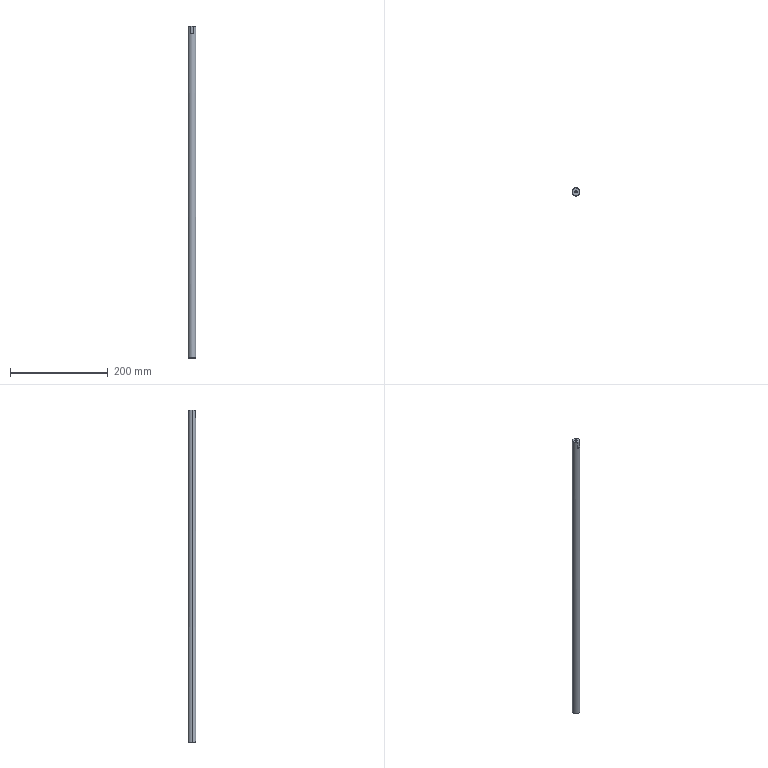Part | STEP file | Support Shaft | 1 solid | 17 faces | box 16 x 16 x 680 mm | volume 136250 mm3 | cone 7 | plane 6 | cylinder 4 | commonest cylinder face diameters 5 x2 16 x2
STEP:
#1=CARTESIAN_POINT('',(0.,0.,0.));
#2=DIRECTION('',(0.,0.,1.));
#3=DIRECTION('',(1.,0.,0.));
#4=AXIS2_PLACEMENT_3D('',#1,#2,#3);
#5=CARTESIAN_POINT('',(-7.5,0.,0.));
#6=VERTEX_POINT('',#5);
#7=CARTESIAN_POINT('',(7.5,0.,0.));
#8=VERTEX_POINT('',#7);
#9=CARTESIAN_POINT('',(0.,0.,0.));
#10=DIRECTION('',(0.,0.,-1.));
#11=DIRECTION('',(1.,0.,0.));
#12=AXIS2_PLACEMENT_3D('',#9,#10,#11);
#13=CIRCLE('',#12,7.5);
#14=CARTESIAN_POINT('',(0.,0.,0.5));
#15=DIRECTION('',(0.,0.,1.));
#16=DIRECTION('',(1.,0.,0.));
#17=AXIS2_PLACEMENT_3D('',#14,#15,#16);
#18=CONICAL_SURFACE('',#17,8.,0.7854);
#19=CARTESIAN_POINT('',(6.283,-0.5));
#20=DIRECTION('',(-1.,0.));
#21=VECTOR('',#20,1.);
#22=LINE('',#19,#21);
#23=(GEOMETRIC_REPRESENTATION_CONTEXT(2)PARAMETRIC_REPRESENTATION_CONTEXT()REPRESENTATION_CONTEXT('',''));
#24=DEFINITIONAL_REPRESENTATION('',(#22),#23);
#25=PCURVE('',#18,#24);
#26=CARTESIAN_POINT('',(0.,0.,0.));
#27=DIRECTION('',(0.,0.,1.));
#28=DIRECTION('',(1.,0.,0.));
#29=AXIS2_PLACEMENT_3D('',#26,#27,#28);
#30=PLANE('',#29);
#31=CARTESIAN_POINT('',(7.5,0.));
#32=CARTESIAN_POINT('',(7.5,-12.99));
#33=CARTESIAN_POINT('',(-3.75,-6.495));
#34=CARTESIAN_POINT('',(-15.,0.));
#35=CARTESIAN_POINT('',(-3.75,6.495));
#36=CARTESIAN_POINT('',(7.5,12.99));
#37=CARTESIAN_POINT('',(7.5,0.));
#38=(BOUNDED_CURVE()B_SPLINE_CURVE(2,(#31,#32,#33,#34,#35,#36,#37),.UNSPECIFIED.,.T.,.F.)B_SPLINE_CURVE_WITH_KNOTS((1,2,2,2,2,1),(-2.094,0.,2.094,4.189,6.283,8.378),.UNSPECIFIED.)CURVE()GEOMETRIC_REPRESENTATION_ITEM()RATIONAL_B_SPLINE_CURVE((1.,0.5,1.,0.5,1.,0.5,1.))REPRESENTATION_ITEM(''));
#39=(GEOMETRIC_REPRESENTATION_CONTEXT(2)PARAMETRIC_REPRESENTATION_CONTEXT()REPRESENTATION_CONTEXT('',''));
#40=DEFINITIONAL_REPRESENTATION('',(#38),#39);
#41=PCURVE('',#30,#40);
#42=SURFACE_CURVE('',#13,(#25,#41),.PCURVE_S1.);
#43=EDGE_CURVE('',#6,#8,#42,.T.);
#44=ORIENTED_EDGE('',*,*,#43,.F.);
#45=CARTESIAN_POINT('',(-8.,0.,0.5));
#46=VERTEX_POINT('',#45);
#47=CARTESIAN_POINT('',(-8.,0.,0.5));
#48=DIRECTION('',(-0.7071,0.,0.7071));
#49=VECTOR('',#48,1.);
#50=LINE('',#47,#49);
#51=CARTESIAN_POINT('',(3.142,0.));
#52=DIRECTION('',(0.,1.));
#53=VECTOR('',#52,1.);
#54=LINE('',#51,#53);
#55=(GEOMETRIC_REPRESENTATION_CONTEXT(2)PARAMETRIC_REPRESENTATION_CONTEXT()REPRESENTATION_CONTEXT('',''));
#56=DEFINITIONAL_REPRESENTATION('',(#54),#55);
#57=PCURVE('',#18,#56);
#58=CARTESIAN_POINT('',(0.,0.,0.5));
#59=DIRECTION('',(0.,0.,1.));
#60=DIRECTION('',(1.,0.,0.));
#61=AXIS2_PLACEMENT_3D('',#58,#59,#60);
#62=CONICAL_SURFACE('',#61,8.,0.7854);
#63=CARTESIAN_POINT('',(3.142,0.));
#64=DIRECTION('',(0.,1.));
#65=VECTOR('',#64,1.);
#66=LINE('',#63,#65);
#67=(GEOMETRIC_REPRESENTATION_CONTEXT(2)PARAMETRIC_REPRESENTATION_CONTEXT()REPRESENTATION_CONTEXT('',''));
#68=DEFINITIONAL_REPRESENTATION('',(#66),#67);
#69=PCURVE('',#62,#68);
#70=SURFACE_CURVE('',#50,(#57,#69),.PCURVE_S1.);
#71=EDGE_CURVE('',#6,#46,#70,.T.);
#72=ORIENTED_EDGE('',*,*,#71,.T.);
#73=CARTESIAN_POINT('',(8.,0.,0.5));
#74=VERTEX_POINT('',#73);
#75=CARTESIAN_POINT('',(0.,0.,0.5));
#76=DIRECTION('',(0.,0.,1.));
#77=DIRECTION('',(1.,0.,0.));
#78=AXIS2_PLACEMENT_3D('',#75,#76,#77);
#79=CIRCLE('',#78,8.);
#80=CARTESIAN_POINT('',(0.,0.));
#81=DIRECTION('',(1.,0.));
#82=VECTOR('',#81,1.);
#83=LINE('',#80,#82);
#84=(GEOMETRIC_REPRESENTATION_CONTEXT(2)PARAMETRIC_REPRESENTATION_CONTEXT()REPRESENTATION_CONTEXT('',''));
#85=DEFINITIONAL_REPRESENTATION('',(#83),#84);
#86=PCURVE('',#18,#85);
#87=CARTESIAN_POINT('',(0.,0.,680.));
#88=DIRECTION('',(0.,0.,-1.));
#89=DIRECTION('',(-1.,0.,0.));
#90=AXIS2_PLACEMENT_3D('',#87,#88,#89);
#91=CYLINDRICAL_SURFACE('',#90,8.);
#92=CARTESIAN_POINT('',(3.142,679.5));
#93=DIRECTION('',(-1.,0.));
#94=VECTOR('',#93,1.);
#95=LINE('',#92,#94);
#96=(GEOMETRIC_REPRESENTATION_CONTEXT(2)PARAMETRIC_REPRESENTATION_CONTEXT()REPRESENTATION_CONTEXT('',''));
#97=DEFINITIONAL_REPRESENTATION('',(#95),#96);
#98=PCURVE('',#91,#97);
#99=SURFACE_CURVE('',#79,(#86,#98),.PCURVE_S1.);
#100=EDGE_CURVE('',#74,#46,#99,.T.);
#101=ORIENTED_EDGE('',*,*,#100,.F.);
#102=CARTESIAN_POINT('',(8.,0.,0.5));
#103=DIRECTION('',(0.7071,0.,0.7071));
#104=VECTOR('',#103,1.);
#105=LINE('',#102,#104);
#106=CARTESIAN_POINT('',(0.,0.));
#107=DIRECTION('',(0.,1.));
#108=VECTOR('',#107,1.);
#109=LINE('',#106,#108);
#110=(GEOMETRIC_REPRESENTATION_CONTEXT(2)PARAMETRIC_REPRESENTATION_CONTEXT()REPRESENTATION_CONTEXT('',''));
#111=DEFINITIONAL_REPRESENTATION('',(#109),#110);
#112=PCURVE('',#18,#111);
#113=CARTESIAN_POINT('',(6.283,0.));
#114=DIRECTION('',(0.,1.));
#115=VECTOR('',#114,1.);
#116=LINE('',#113,#115);
#117=(GEOMETRIC_REPRESENTATION_CONTEXT(2)PARAMETRIC_REPRESENTATION_CONTEXT()REPRESENTATION_CONTEXT('',''));
#118=DEFINITIONAL_REPRESENTATION('',(#116),#117);
#119=PCURVE('',#62,#118);
#120=SURFACE_CURVE('',#105,(#112,#119),.PCURVE_S1.);
#121=EDGE_CURVE('',#8,#74,#120,.T.);
#122=ORIENTED_EDGE('',*,*,#121,.F.);
#123=EDGE_LOOP('',(#44,#72,#101,#122));
#124=FACE_BOUND('',#123,.T.);
#125=ADVANCED_FACE('',(#124),#18,.T.);
#126=CARTESIAN_POINT('',(2.5,0.,665.));
#127=VERTEX_POINT('',#126);
#128=CARTESIAN_POINT('',(2.5,0.,680.));
#129=VERTEX_POINT('',#128);
#130=CARTESIAN_POINT('',(2.5,0.,680.));
#131=DIRECTION('',(0.,0.,1.));
#132=VECTOR('',#131,1.);
#133=LINE('',#130,#132);
#134=CARTESIAN_POINT('',(0.,0.,680.));
#135=DIRECTION('',(0.,0.,1.));
#136=DIRECTION('',(1.,0.,0.));
#137=AXIS2_PLACEMENT_3D('',#134,#135,#136);
#138=CYLINDRICAL_SURFACE('',#137,2.5);
#139=CARTESIAN_POINT('',(6.283,0.));
#140=DIRECTION('',(0.,1.));
#141=VECTOR('',#140,1.);
#142=LINE('',#139,#141);
#143=(GEOMETRIC_REPRESENTATION_CONTEXT(2)PARAMETRIC_REPRESENTATION_CONTEXT()REPRESENTATION_CONTEXT('',''));
#144=DEFINITIONAL_REPRESENTATION('',(#142),#143);
#145=PCURVE('',#138,#144);
#146=CARTESIAN_POINT('',(0.,0.,680.));
#147=DIRECTION('',(0.,0.,1.));
#148=DIRECTION('',(1.,0.,0.));
#149=AXIS2_PLACEMENT_3D('',#146,#147,#148);
#150=CYLINDRICAL_SURFACE('',#149,2.5);
#151=CARTESIAN_POINT('',(0.,0.));
#152=DIRECTION('',(0.,1.));
#153=VECTOR('',#152,1.);
#154=LINE('',#151,#153);
#155=(GEOMETRIC_REPRESENTATION_CONTEXT(2)PARAMETRIC_REPRESENTATION_CONTEXT()REPRESENTATION_CONTEXT('',''));
#156=DEFINITIONAL_REPRESENTATION('',(#154),#155);
#157=PCURVE('',#150,#156);
#158=SURFACE_CURVE('',#133,(#145,#157),.PCURVE_S1.);
#159=EDGE_CURVE('',#127,#129,#158,.T.);
#160=ORIENTED_EDGE('',*,*,#159,.T.);
#161=CARTESIAN_POINT('',(-2.5,0.,680.));
#162=VERTEX_POINT('',#161);
#163=CARTESIAN_POINT('',(0.,0.,680.));
#164=DIRECTION('',(0.,0.,1.));
#165=DIRECTION('',(1.,0.,0.));
#166=AXIS2_PLACEMENT_3D('',#163,#164,#165);
#167=CIRCLE('',#166,2.5);
#168=CARTESIAN_POINT('',(0.,0.));
#169=DIRECTION('',(1.,0.));
#170=VECTOR('',#169,1.);
#171=LINE('',#168,#170);
#172=(GEOMETRIC_REPRESENTATION_CONTEXT(2)PARAMETRIC_REPRESENTATION_CONTEXT()REPRESENTATION_CONTEXT('',''));
#173=DEFINITIONAL_REPRESENTATION('',(#171),#172);
#174=PCURVE('',#138,#173);
#175=CARTESIAN_POINT('',(0.,0.,680.));
#176=DIRECTION('',(0.,0.,1.));
#177=DIRECTION('',(1.,0.,0.));
#178=AXIS2_PLACEMENT_3D('',#175,#176,#177);
#179=PLANE('',#178);
#180=CARTESIAN_POINT('',(0.,0.));
#181=DIRECTION('',(1.,0.));
#182=AXIS2_PLACEMENT_2D('',#180,#181);
#183=CIRCLE('',#182,2.5);
#184=(GEOMETRIC_REPRESENTATION_CONTEXT(2)PARAMETRIC_REPRESENTATION_CONTEXT()REPRESENTATION_CONTEXT('',''));
#185=DEFINITIONAL_REPRESENTATION('',(#183),#184);
#186=PCURVE('',#179,#185);
#187=SURFACE_CURVE('',#167,(#174,#186),.PCURVE_S1.);
#188=EDGE_CURVE('',#162,#129,#187,.T.);
#189=ORIENTED_EDGE('',*,*,#188,.F.);
#190=CARTESIAN_POINT('',(-2.5,0.,665.));
#191=VERTEX_POINT('',#190);
#192=CARTESIAN_POINT('',(-2.5,0.,680.));
#193=DIRECTION('',(0.,0.,1.));
#194=VECTOR('',#193,1.);
#195=LINE('',#192,#194);
#196=CARTESIAN_POINT('',(3.142,0.));
#197=DIRECTION('',(0.,1.));
#198=VECTOR('',#197,1.);
#199=LINE('',#196,#198);
#200=(GEOMETRIC_REPRESENTATION_CONTEXT(2)PARAMETRIC_REPRESENTATION_CONTEXT()REPRESENTATION_CONTEXT('',''));
#201=DEFINITIONAL_REPRESENTATION('',(#199),#200);
#202=PCURVE('',#138,#201);
#203=CARTESIAN_POINT('',(3.142,0.));
#204=DIRECTION('',(0.,1.));
#205=VECTOR('',#204,1.);
#206=LINE('',#203,#205);
#207=(GEOMETRIC_REPRESENTATION_CONTEXT(2)PARAMETRIC_REPRESENTATION_CONTEXT()REPRESENTATION_CONTEXT('',''));
#208=DEFINITIONAL_REPRESENTATION('',(#206),#207);
#209=PCURVE('',#150,#208);
#210=SURFACE_CURVE('',#195,(#202,#209),.PCURVE_S1.);
#211=EDGE_CURVE('',#191,#162,#210,.T.);
#212=ORIENTED_EDGE('',*,*,#211,.F.);
#213=CARTESIAN_POINT('',(0.,0.,665.));
#214=DIRECTION('',(0.,0.,1.));
#215=DIRECTION('',(1.,0.,0.));
#216=AXIS2_PLACEMENT_3D('',#213,#214,#215);
#217=CIRCLE('',#216,2.5);
#218=CARTESIAN_POINT('',(0.,-15.));
#219=DIRECTION('',(1.,0.));
#220=VECTOR('',#219,1.);
#221=LINE('',#218,#220);
#222=(GEOMETRIC_REPRESENTATION_CONTEXT(2)PARAMETRIC_REPRESENTATION_CONTEXT()REPRESENTATION_CONTEXT('',''));
#223=DEFINITIONAL_REPRESENTATION('',(#221),#222);
#224=PCURVE('',#138,#223);
#225=CARTESIAN_POINT('',(0.,0.,665.));
#226=DIRECTION('',(0.,0.,1.));
#227=DIRECTION('',(1.,0.,0.));
#228=AXIS2_PLACEMENT_3D('',#225,#226,#227);
#229=CONICAL_SURFACE('',#228,2.5,1.03);
#230=CARTESIAN_POINT('',(0.,0.));
#231=DIRECTION('',(1.,0.));
#232=VECTOR('',#231,1.);
#233=LINE('',#230,#232);
#234=(GEOMETRIC_REPRESENTATION_CONTEXT(2)PARAMETRIC_REPRESENTATION_CONTEXT()REPRESENTATION_CONTEXT('',''));
#235=DEFINITIONAL_REPRESENTATION('',(#233),#234);
#236=PCURVE('',#229,#235);
#237=SURFACE_CURVE('',#217,(#224,#236),.PCURVE_S1.);
#238=EDGE_CURVE('',#191,#127,#237,.T.);
#239=ORIENTED_EDGE('',*,*,#238,.T.);
#240=EDGE_LOOP('',(#160,#189,#212,#239));
#241=FACE_BOUND('',#240,.F.);
#242=ADVANCED_FACE('',(#241),#138,.F.);
#243=ORIENTED_EDGE('',*,*,#238,.F.);
#244=CARTESIAN_POINT('',(0.,0.,663.498));
#245=VERTEX_POINT('',#244);
#246=CARTESIAN_POINT('',(-2.5,0.,665.));
#247=DIRECTION('',(-0.8572,0.,0.515));
#248=VECTOR('',#247,1.);
#249=LINE('',#246,#248);
#250=CARTESIAN_POINT('',(3.142,0.));
#251=DIRECTION('',(0.,1.));
#252=VECTOR('',#251,1.);
#253=LINE('',#250,#252);
#254=(GEOMETRIC_REPRESENTATION_CONTEXT(2)PARAMETRIC_REPRESENTATION_CONTEXT()REPRESENTATION_CONTEXT('',''));
#255=DEFINITIONAL_REPRESENTATION('',(#253),#254);
#256=PCURVE('',#229,#255);
#257=CARTESIAN_POINT('',(0.,0.,665.));
#258=DIRECTION('',(0.,0.,1.));
#259=DIRECTION('',(1.,0.,0.));
#260=AXIS2_PLACEMENT_3D('',#257,#258,#259);
#261=CONICAL_SURFACE('',#260,2.5,1.03);
#262=CARTESIAN_POINT('',(3.142,0.));
#263=DIRECTION('',(0.,1.));
#264=VECTOR('',#263,1.);
#265=LINE('',#262,#264);
#266=(GEOMETRIC_REPRESENTATION_CONTEXT(2)PARAMETRIC_REPRESENTATION_CONTEXT()REPRESENTATION_CONTEXT('',''));
#267=DEFINITIONAL_REPRESENTATION('',(#265),#266);
#268=PCURVE('',#261,#267);
#269=SURFACE_CURVE('',#249,(#256,#268),.PCURVE_S1.);
#270=EDGE_CURVE('',#245,#191,#269,.T.);
#271=ORIENTED_EDGE('',*,*,#270,.F.);
#272=CARTESIAN_POINT('',(2.5,0.,665.));
#273=DIRECTION('',(0.8572,0.,0.515));
#274=VECTOR('',#273,1.);
#275=LINE('',#272,#274);
#276=CARTESIAN_POINT('',(6.283,0.));
#277=DIRECTION('',(0.,1.));
#278=VECTOR('',#277,1.);
#279=LINE('',#276,#278);
#280=(GEOMETRIC_REPRESENTATION_CONTEXT(2)PARAMETRIC_REPRESENTATION_CONTEXT()REPRESENTATION_CONTEXT('',''));
#281=DEFINITIONAL_REPRESENTATION('',(#279),#280);
#282=PCURVE('',#229,#281);
#283=CARTESIAN_POINT('',(0.,0.));
#284=DIRECTION('',(0.,1.));
#285=VECTOR('',#284,1.);
#286=LINE('',#283,#285);
#287=(GEOMETRIC_REPRESENTATION_CONTEXT(2)PARAMETRIC_REPRESENTATION_CONTEXT()REPRESENTATION_CONTEXT('',''));
#288=DEFINITIONAL_REPRESENTATION('',(#286),#287);
#289=PCURVE('',#261,#288);
#290=SURFACE_CURVE('',#275,(#282,#289),.PCURVE_S1.);
#291=EDGE_CURVE('',#245,#127,#290,.T.);
#292=ORIENTED_EDGE('',*,*,#291,.T.);
#293=EDGE_LOOP('',(#243,#271,#292));
#294=FACE_BOUND('',#293,.F.);
#295=ADVANCED_FACE('',(#294),#229,.F.);
#296=CARTESIAN_POINT('',(-7.5,0.,680.));
#297=VERTEX_POINT('',#296);
#298=CARTESIAN_POINT('',(-2.693,-7.,680.));
#299=VERTEX_POINT('',#298);
#300=CARTESIAN_POINT('',(0.,0.,680.));
#301=DIRECTION('',(0.,0.,1.));
#302=DIRECTION('',(1.,0.,0.));
#303=AXIS2_PLACEMENT_3D('',#300,#301,#302);
#304=CIRCLE('',#303,7.5);
#305=CARTESIAN_POINT('',(0.,0.,680.));
#306=DIRECTION('',(0.,0.,-1.));
#307=DIRECTION('',(-1.,0.,0.));
#308=AXIS2_PLACEMENT_3D('',#305,#306,#307);
#309=CONICAL_SURFACE('',#308,7.5,0.7854);
#310=CARTESIAN_POINT('',(9.425,0.));
#311=DIRECTION('',(-1.,0.));
#312=VECTOR('',#311,1.);
#313=LINE('',#310,#312);
#314=(GEOMETRIC_REPRESENTATION_CONTEXT(2)PARAMETRIC_REPRESENTATION_CONTEXT()REPRESENTATION_CONTEXT('',''));
#315=DEFINITIONAL_REPRESENTATION('',(#313),#314);
#316=PCURVE('',#309,#315);
#317=CARTESIAN_POINT('',(0.,0.));
#318=DIRECTION('',(1.,0.));
#319=AXIS2_PLACEMENT_2D('',#317,#318);
#320=CIRCLE('',#319,7.5);
#321=(GEOMETRIC_REPRESENTATION_CONTEXT(2)PARAMETRIC_REPRESENTATION_CONTEXT()REPRESENTATION_CONTEXT('',''));
#322=DEFINITIONAL_REPRESENTATION('',(#320),#321);
#323=PCURVE('',#179,#322);
#324=SURFACE_CURVE('',#304,(#316,#323),.PCURVE_S1.);
#325=EDGE_CURVE('',#297,#299,#324,.T.);
#326=ORIENTED_EDGE('',*,*,#325,.F.);
#327=CARTESIAN_POINT('',(-8.,0.,679.5));
#328=VERTEX_POINT('',#327);
#329=CARTESIAN_POINT('',(-7.5,0.,680.));
#330=DIRECTION('',(-0.7071,0.,-0.7071));
#331=VECTOR('',#330,1.);
#332=LINE('',#329,#331);
#333=CARTESIAN_POINT('',(6.283,0.));
#334=DIRECTION('',(0.,1.));
#335=VECTOR('',#334,1.);
#336=LINE('',#333,#335);
#337=(GEOMETRIC_REPRESENTATION_CONTEXT(2)PARAMETRIC_REPRESENTATION_CONTEXT()REPRESENTATION_CONTEXT('',''));
#338=DEFINITIONAL_REPRESENTATION('',(#336),#337);
#339=PCURVE('',#309,#338);
#340=CARTESIAN_POINT('',(0.,0.,680.));
#341=DIRECTION('',(0.,0.,-1.));
#342=DIRECTION('',(-1.,0.,0.));
#343=AXIS2_PLACEMENT_3D('',#340,#341,#342);
#344=CONICAL_SURFACE('',#343,7.5,0.7854);
#345=CARTESIAN_POINT('',(0.,0.));
#346=DIRECTION('',(0.,1.));
#347=VECTOR('',#346,1.);
#348=LINE('',#345,#347);
#349=(GEOMETRIC_REPRESENTATION_CONTEXT(2)PARAMETRIC_REPRESENTATION_CONTEXT()REPRESENTATION_CONTEXT('',''));
#350=DEFINITIONAL_REPRESENTATION('',(#348),#349);
#351=PCURVE('',#344,#350);
#352=SURFACE_CURVE('',#332,(#339,#351),.PCURVE_S1.);
#353=EDGE_CURVE('',#297,#328,#352,.T.);
#354=ORIENTED_EDGE('',*,*,#353,.T.);
#355=CARTESIAN_POINT('',(-3.873,-7.,679.5));
#356=VERTEX_POINT('',#355);
#357=CARTESIAN_POINT('',(0.,0.,679.5));
#358=DIRECTION('',(0.,0.,-1.));
#359=DIRECTION('',(1.,0.,0.));
#360=AXIS2_PLACEMENT_3D('',#357,#358,#359);
#361=CIRCLE('',#360,8.);
#362=CARTESIAN_POINT('',(3.142,0.5));
#363=DIRECTION('',(1.,0.));
#364=VECTOR('',#363,1.);
#365=LINE('',#362,#364);
#366=(GEOMETRIC_REPRESENTATION_CONTEXT(2)PARAMETRIC_REPRESENTATION_CONTEXT()REPRESENTATION_CONTEXT('',''));
#367=DEFINITIONAL_REPRESENTATION('',(#365),#366);
#368=PCURVE('',#309,#367);
#369=CARTESIAN_POINT('',(0.,0.,680.));
#370=DIRECTION('',(0.,0.,-1.));
#371=DIRECTION('',(-1.,0.,0.));
#372=AXIS2_PLACEMENT_3D('',#369,#370,#371);
#373=CYLINDRICAL_SURFACE('',#372,8.);
#374=CARTESIAN_POINT('',(3.142,0.5));
#375=DIRECTION('',(1.,0.));
#376=VECTOR('',#375,1.);
#377=LINE('',#374,#376);
#378=(GEOMETRIC_REPRESENTATION_CONTEXT(2)PARAMETRIC_REPRESENTATION_CONTEXT()REPRESENTATION_CONTEXT('',''));
#379=DEFINITIONAL_REPRESENTATION('',(#377),#378);
#380=PCURVE('',#373,#379);
#381=SURFACE_CURVE('',#361,(#368,#380),.PCURVE_S1.);
#382=EDGE_CURVE('',#356,#328,#381,.T.);
#383=ORIENTED_EDGE('',*,*,#382,.F.);
#384=CARTESIAN_POINT('',(-3.873,-7.,679.5));
#385=CARTESIAN_POINT('',(-3.488,-7.,679.686));
#386=CARTESIAN_POINT('',(-3.096,-7.,679.855));
#387=CARTESIAN_POINT('',(-2.693,-7.,680.));
#388=B_SPLINE_CURVE_WITH_KNOTS('',3,(#384,#385,#386,#387),.UNSPECIFIED.,.F.,.F.,(4,4),(0.01564,0.01692),.PIECEWISE_BEZIER_KNOTS.);
#389=CARTESIAN_POINT('',(5.218,0.5));
#390=CARTESIAN_POINT('',(5.216,0.4915));
#391=CARTESIAN_POINT('',(5.212,0.4747));
#392=CARTESIAN_POINT('',(5.206,0.4496));
#393=CARTESIAN_POINT('',(5.2,0.4248));
#394=CARTESIAN_POINT('',(5.194,0.4002));
#395=CARTESIAN_POINT('',(5.188,0.3758));
#396=CARTESIAN_POINT('',(5.182,0.3516));
#397=CARTESIAN_POINT('',(5.176,0.3277));
#398=CARTESIAN_POINT('',(5.17,0.304));
#399=CARTESIAN_POINT('',(5.164,0.2806));
#400=CARTESIAN_POINT('',(5.158,0.2574));
#401=CARTESIAN_POINT('',(5.152,0.2345));
#402=CARTESIAN_POINT('',(5.145,0.2118));
#403=CARTESIAN_POINT('',(5.139,0.1894));
#404=CARTESIAN_POINT('',(5.133,0.1672));
#405=CARTESIAN_POINT('',(5.126,0.1453));
#406=CARTESIAN_POINT('',(5.12,0.1237));
#407=CARTESIAN_POINT('',(5.113,0.1024));
#408=CARTESIAN_POINT('',(5.107,0.08131));
#409=CARTESIAN_POINT('',(5.1,0.06053));
#410=CARTESIAN_POINT('',(5.093,0.04005));
#411=CARTESIAN_POINT('',(5.086,0.01985));
#412=CARTESIAN_POINT('',(5.082,0.006583));
#413=CARTESIAN_POINT('',(5.08,0.));
#414=B_SPLINE_CURVE_WITH_KNOTS('',3,(#389,#390,#391,#392,#393,#394,#395,#396,#397,#398,#399,#400,#401,#402,#403,#404,#405,#406,#407,#408,#409,#410,#411,#412,#413),.UNSPECIFIED.,.F.,.F.,(4,1,1,1,1,1,1,1,1,1,1,1,1,1,1,1,1,1,1,1,1,1,4),(0.01564,0.01569,0.01575,0.01581,0.01587,0.01593,0.01599,0.01604,0.0161,0.01616,0.01622,0.01628,0.01634,0.01639,0.01645,0.01651,0.01657,0.01663,0.01669,0.01674,0.0168,0.01686,0.01692),.QUASI_UNIFORM_KNOTS.);
#415=(GEOMETRIC_REPRESENTATION_CONTEXT(2)PARAMETRIC_REPRESENTATION_CONTEXT()REPRESENTATION_CONTEXT('',''));
#416=DEFINITIONAL_REPRESENTATION('',(#414),#415);
#417=PCURVE('',#309,#416);
#418=CARTESIAN_POINT('',(-10.766,-7.,665.));
#419=DIRECTION('',(0.,-1.,0.));
#420=DIRECTION('',(0.,0.,-1.));
#421=AXIS2_PLACEMENT_3D('',#418,#419,#420);
#422=PLANE('',#421);
#423=CARTESIAN_POINT('',(-14.5,6.893));
#424=CARTESIAN_POINT('',(-14.686,7.278));
#425=CARTESIAN_POINT('',(-14.855,7.67));
#426=CARTESIAN_POINT('',(-15.,8.074));
#427=B_SPLINE_CURVE_WITH_KNOTS('',3,(#423,#424,#425,#426),.UNSPECIFIED.,.F.,.F.,(4,4),(0.01564,0.01692),.PIECEWISE_BEZIER_KNOTS.);
#428=(GEOMETRIC_REPRESENTATION_CONTEXT(2)PARAMETRIC_REPRESENTATION_CONTEXT()REPRESENTATION_CONTEXT('',''));
#429=DEFINITIONAL_REPRESENTATION('',(#427),#428);
#430=PCURVE('',#422,#429);
#431=SURFACE_CURVE('',#388,(#417,#430),.PCURVE_S1.);
#432=EDGE_CURVE('',#356,#299,#431,.T.);
#433=ORIENTED_EDGE('',*,*,#432,.T.);
#434=EDGE_LOOP('',(#326,#354,#383,#433));
#435=FACE_BOUND('',#434,.T.);
#436=ADVANCED_FACE('',(#435),#309,.T.);
#437=CARTESIAN_POINT('',(3.873,7.,679.5));
#438=VERTEX_POINT('',#437);
#439=CARTESIAN_POINT('',(8.,0.,679.5));
#440=VERTEX_POINT('',#439);
#441=CARTESIAN_POINT('',(0.,0.,679.5));
#442=DIRECTION('',(0.,0.,-1.));
#443=DIRECTION('',(1.,0.,0.));
#444=AXIS2_PLACEMENT_3D('',#441,#442,#443);
#445=CIRCLE('',#444,8.);
#446=CARTESIAN_POINT('',(-3.142,0.5));
#447=DIRECTION('',(1.,0.));
#448=VECTOR('',#447,1.);
#449=LINE('',#446,#448);
#450=(GEOMETRIC_REPRESENTATION_CONTEXT(2)PARAMETRIC_REPRESENTATION_CONTEXT()REPRESENTATION_CONTEXT('',''));
#451=DEFINITIONAL_REPRESENTATION('',(#449),#450);
#452=PCURVE('',#91,#451);
#453=CARTESIAN_POINT('',(0.,0.,680.));
#454=DIRECTION('',(0.,0.,-1.));
#455=DIRECTION('',(-1.,0.,0.));
#456=AXIS2_PLACEMENT_3D('',#453,#454,#455);
#457=CONICAL_SURFACE('',#456,7.5,0.7854);
#458=CARTESIAN_POINT('',(-3.142,0.5));
#459=DIRECTION('',(1.,0.));
#460=VECTOR('',#459,1.);
#461=LINE('',#458,#460);
#462=(GEOMETRIC_REPRESENTATION_CONTEXT(2)PARAMETRIC_REPRESENTATION_CONTEXT()REPRESENTATION_CONTEXT('',''));
#463=DEFINITIONAL_REPRESENTATION('',(#461),#462);
#464=PCURVE('',#457,#463);
#465=SURFACE_CURVE('',#445,(#452,#464),.PCURVE_S1.);
#466=EDGE_CURVE('',#438,#440,#465,.T.);
#467=ORIENTED_EDGE('',*,*,#466,.T.);
#468=CARTESIAN_POINT('',(8.,0.,680.));
#469=DIRECTION('',(0.,0.,-1.));
#470=VECTOR('',#469,1.);
#471=LINE('',#468,#470);
#472=CARTESIAN_POINT('',(3.142,0.));
#473=DIRECTION('',(0.,1.));
#474=VECTOR('',#473,1.);
#475=LINE('',#472,#474);
#476=(GEOMETRIC_REPRESENTATION_CONTEXT(2)PARAMETRIC_REPRESENTATION_CONTEXT()REPRESENTATION_CONTEXT('',''));
#477=DEFINITIONAL_REPRESENTATION('',(#475),#476);
#478=PCURVE('',#91,#477);
#479=CARTESIAN_POINT('',(3.142,0.));
#480=DIRECTION('',(0.,1.));
#481=VECTOR('',#480,1.);
#482=LINE('',#479,#481);
#483=(GEOMETRIC_REPRESENTATION_CONTEXT(2)PARAMETRIC_REPRESENTATION_CONTEXT()REPRESENTATION_CONTEXT('',''));
#484=DEFINITIONAL_REPRESENTATION('',(#482),#483);
#485=PCURVE('',#373,#484);
#486=SURFACE_CURVE('',#471,(#478,#485),.PCURVE_S1.);
#487=EDGE_CURVE('',#440,#74,#486,.T.);
#488=ORIENTED_EDGE('',*,*,#487,.T.);
#489=ORIENTED_EDGE('',*,*,#100,.T.);
#490=CARTESIAN_POINT('',(-8.,0.,680.));
#491=DIRECTION('',(0.,0.,-1.));
#492=VECTOR('',#491,1.);
#493=LINE('',#490,#492);
#494=CARTESIAN_POINT('',(0.,0.));
#495=DIRECTION('',(0.,1.));
#496=VECTOR('',#495,1.);
#497=LINE('',#494,#496);
#498=(GEOMETRIC_REPRESENTATION_CONTEXT(2)PARAMETRIC_REPRESENTATION_CONTEXT()REPRESENTATION_CONTEXT('',''));
#499=DEFINITIONAL_REPRESENTATION('',(#497),#498);
#500=PCURVE('',#91,#499);
#501=CARTESIAN_POINT('',(6.283,0.));
#502=DIRECTION('',(0.,1.));
#503=VECTOR('',#502,1.);
#504=LINE('',#501,#503);
#505=(GEOMETRIC_REPRESENTATION_CONTEXT(2)PARAMETRIC_REPRESENTATION_CONTEXT()REPRESENTATION_CONTEXT('',''));
#506=DEFINITIONAL_REPRESENTATION('',(#504),#505);
#507=PCURVE('',#373,#506);
#508=SURFACE_CURVE('',#493,(#500,#507),.PCURVE_S1.);
#509=EDGE_CURVE('',#328,#46,#508,.T.);
#510=ORIENTED_EDGE('',*,*,#509,.F.);
#511=CARTESIAN_POINT('',(-3.873,7.,679.5));
#512=VERTEX_POINT('',#511);
#513=CARTESIAN_POINT('',(0.,0.,679.5));
#514=DIRECTION('',(0.,0.,-1.));
#515=DIRECTION('',(1.,0.,0.));
#516=AXIS2_PLACEMENT_3D('',#513,#514,#515);
#517=CIRCLE('',#516,8.);
#518=CARTESIAN_POINT('',(-3.142,0.5));
#519=DIRECTION('',(1.,0.));
#520=VECTOR('',#519,1.);
#521=LINE('',#518,#520);
#522=(GEOMETRIC_REPRESENTATION_CONTEXT(2)PARAMETRIC_REPRESENTATION_CONTEXT()REPRESENTATION_CONTEXT('',''));
#523=DEFINITIONAL_REPRESENTATION('',(#521),#522);
#524=PCURVE('',#91,#523);
#525=CARTESIAN_POINT('',(-3.142,0.5));
#526=DIRECTION('',(1.,0.));
#527=VECTOR('',#526,1.);
#528=LINE('',#525,#527);
#529=(GEOMETRIC_REPRESENTATION_CONTEXT(2)PARAMETRIC_REPRESENTATION_CONTEXT()REPRESENTATION_CONTEXT('',''));
#530=DEFINITIONAL_REPRESENTATION('',(#528),#529);
#531=PCURVE('',#344,#530);
#532=SURFACE_CURVE('',#517,(#524,#531),.PCURVE_S1.);
#533=EDGE_CURVE('',#328,#512,#532,.T.);
#534=ORIENTED_EDGE('',*,*,#533,.T.);
#535=CARTESIAN_POINT('',(-3.873,7.,665.));
#536=VERTEX_POINT('',#535);
#537=CARTESIAN_POINT('',(-3.873,7.,680.));
#538=DIRECTION('',(0.,0.,1.));
#539=VECTOR('',#538,1.);
#540=LINE('',#537,#539);
#541=CARTESIAN_POINT('',(1.065,0.));
#542=DIRECTION('',(0.,-1.));
#543=VECTOR('',#542,1.);
#544=LINE('',#541,#543);
#545=(GEOMETRIC_REPRESENTATION_CONTEXT(2)PARAMETRIC_REPRESENTATION_CONTEXT()REPRESENTATION_CONTEXT('',''));
#546=DEFINITIONAL_REPRESENTATION('',(#544),#545);
#547=PCURVE('',#91,#546);
#548=CARTESIAN_POINT('',(-10.766,7.,665.));
#549=DIRECTION('',(0.,1.,0.));
#550=DIRECTION('',(0.,0.,1.));
#551=AXIS2_PLACEMENT_3D('',#548,#549,#550);
#552=PLANE('',#551);
#553=CARTESIAN_POINT('',(15.,6.893));
#554=DIRECTION('',(1.,0.));
#555=VECTOR('',#554,1.);
#556=LINE('',#553,#555);
#557=(GEOMETRIC_REPRESENTATION_CONTEXT(2)PARAMETRIC_REPRESENTATION_CONTEXT()REPRESENTATION_CONTEXT('',''));
#558=DEFINITIONAL_REPRESENTATION('',(#556),#557);
#559=PCURVE('',#552,#558);
#560=SURFACE_CURVE('',#540,(#547,#559),.PCURVE_S1.);
#561=EDGE_CURVE('',#536,#512,#560,.T.);
#562=ORIENTED_EDGE('',*,*,#561,.F.);
#563=CARTESIAN_POINT('',(3.873,7.,665.));
#564=VERTEX_POINT('',#563);
#565=CARTESIAN_POINT('',(0.,0.,665.));
#566=DIRECTION('',(0.,0.,1.));
#567=DIRECTION('',(1.,0.,0.));
#568=AXIS2_PLACEMENT_3D('',#565,#566,#567);
#569=CIRCLE('',#568,8.);
#570=CARTESIAN_POINT('',(3.142,15.));
#571=DIRECTION('',(-1.,0.));
#572=VECTOR('',#571,1.);
#573=LINE('',#570,#572);
#574=(GEOMETRIC_REPRESENTATION_CONTEXT(2)PARAMETRIC_REPRESENTATION_CONTEXT()REPRESENTATION_CONTEXT('',''));
#575=DEFINITIONAL_REPRESENTATION('',(#573),#574);
#576=PCURVE('',#91,#575);
#577=CARTESIAN_POINT('',(0.,0.,665.));
#578=DIRECTION('',(0.,0.,1.));
#579=DIRECTION('',(1.,0.,0.));
#580=AXIS2_PLACEMENT_3D('',#577,#578,#579);
#581=PLANE('',#580);
#582=CARTESIAN_POINT('',(0.,0.));
#583=DIRECTION('',(1.,0.));
#584=AXIS2_PLACEMENT_2D('',#582,#583);
#585=CIRCLE('',#584,8.);
#586=(GEOMETRIC_REPRESENTATION_CONTEXT(2)PARAMETRIC_REPRESENTATION_CONTEXT()REPRESENTATION_CONTEXT('',''));
#587=DEFINITIONAL_REPRESENTATION('',(#585),#586);
#588=PCURVE('',#581,#587);
#589=SURFACE_CURVE('',#569,(#576,#588),.PCURVE_S1.);
#590=EDGE_CURVE('',#564,#536,#589,.T.);
#591=ORIENTED_EDGE('',*,*,#590,.F.);
#592=CARTESIAN_POINT('',(3.873,7.,680.));
#593=DIRECTION('',(0.,0.,-1.));
#594=VECTOR('',#593,1.);
#595=LINE('',#592,#594);
#596=CARTESIAN_POINT('',(2.076,0.));
#597=DIRECTION('',(0.,1.));
#598=VECTOR('',#597,1.);
#599=LINE('',#596,#598);
#600=(GEOMETRIC_REPRESENTATION_CONTEXT(2)PARAMETRIC_REPRESENTATION_CONTEXT()REPRESENTATION_CONTEXT('',''));
#601=DEFINITIONAL_REPRESENTATION('',(#599),#600);
#602=PCURVE('',#91,#601);
#603=CARTESIAN_POINT('',(15.,14.639));
#604=DIRECTION('',(-1.,0.));
#605=VECTOR('',#604,1.);
#606=LINE('',#603,#605);
#607=(GEOMETRIC_REPRESENTATION_CONTEXT(2)PARAMETRIC_REPRESENTATION_CONTEXT()REPRESENTATION_CONTEXT('',''));
#608=DEFINITIONAL_REPRESENTATION('',(#606),#607);
#609=PCURVE('',#552,#608);
#610=SURFACE_CURVE('',#595,(#602,#609),.PCURVE_S1.);
#611=EDGE_CURVE('',#438,#564,#610,.T.);
#612=ORIENTED_EDGE('',*,*,#611,.F.);
#613=EDGE_LOOP('',(#467,#488,#489,#510,#534,#562,#591,#612));
#614=FACE_BOUND('',#613,.T.);
#615=ADVANCED_FACE('',(#614),#91,.T.);
#616=ORIENTED_EDGE('',*,*,#487,.F.);
#617=CARTESIAN_POINT('',(3.873,-7.,679.5));
#618=VERTEX_POINT('',#617);
#619=CARTESIAN_POINT('',(0.,0.,679.5));
#620=DIRECTION('',(0.,0.,-1.));
#621=DIRECTION('',(1.,0.,0.));
#622=AXIS2_PLACEMENT_3D('',#619,#620,#621);
#623=CIRCLE('',#622,8.);
#624=CARTESIAN_POINT('',(3.142,0.5));
#625=DIRECTION('',(1.,0.));
#626=VECTOR('',#625,1.);
#627=LINE('',#624,#626);
#628=(GEOMETRIC_REPRESENTATION_CONTEXT(2)PARAMETRIC_REPRESENTATION_CONTEXT()REPRESENTATION_CONTEXT('',''));
#629=DEFINITIONAL_REPRESENTATION('',(#627),#628);
#630=PCURVE('',#373,#629);
#631=CARTESIAN_POINT('',(3.142,0.5));
#632=DIRECTION('',(1.,0.));
#633=VECTOR('',#632,1.);
#634=LINE('',#631,#633);
#635=(GEOMETRIC_REPRESENTATION_CONTEXT(2)PARAMETRIC_REPRESENTATION_CONTEXT()REPRESENTATION_CONTEXT('',''));
#636=DEFINITIONAL_REPRESENTATION('',(#634),#635);
#637=PCURVE('',#457,#636);
#638=SURFACE_CURVE('',#623,(#630,#637),.PCURVE_S1.);
#639=EDGE_CURVE('',#440,#618,#638,.T.);
#640=ORIENTED_EDGE('',*,*,#639,.T.);
#641=CARTESIAN_POINT('',(3.873,-7.,665.));
#642=VERTEX_POINT('',#641);
#643=CARTESIAN_POINT('',(3.873,-7.,680.));
#644=DIRECTION('',(0.,0.,1.));
#645=VECTOR('',#644,1.);
#646=LINE('',#643,#645);
#647=CARTESIAN_POINT('',(4.207,0.));
#648=DIRECTION('',(0.,-1.));
#649=VECTOR('',#648,1.);
#650=LINE('',#647,#649);
#651=(GEOMETRIC_REPRESENTATION_CONTEXT(2)PARAMETRIC_REPRESENTATION_CONTEXT()REPRESENTATION_CONTEXT('',''));
#652=DEFINITIONAL_REPRESENTATION('',(#650),#651);
#653=PCURVE('',#373,#652);
#654=CARTESIAN_POINT('',(-15.,14.639));
#655=DIRECTION('',(-1.,0.));
#656=VECTOR('',#655,1.);
#657=LINE('',#654,#656);
#658=(GEOMETRIC_REPRESENTATION_CONTEXT(2)PARAMETRIC_REPRESENTATION_CONTEXT()REPRESENTATION_CONTEXT('',''));
#659=DEFINITIONAL_REPRESENTATION('',(#657),#658);
#660=PCURVE('',#422,#659);
#661=SURFACE_CURVE('',#646,(#653,#660),.PCURVE_S1.);
#662=EDGE_CURVE('',#642,#618,#661,.T.);
#663=ORIENTED_EDGE('',*,*,#662,.F.);
#664=CARTESIAN_POINT('',(-3.873,-7.,665.));
#665=VERTEX_POINT('',#664);
#666=CARTESIAN_POINT('',(0.,0.,665.));
#667=DIRECTION('',(0.,0.,1.));
#668=DIRECTION('',(1.,0.,0.));
#669=AXIS2_PLACEMENT_3D('',#666,#667,#668);
#670=CIRCLE('',#669,8.);
#671=CARTESIAN_POINT('',(9.425,15.));
#672=DIRECTION('',(-1.,0.));
#673=VECTOR('',#672,1.);
#674=LINE('',#671,#673);
#675=(GEOMETRIC_REPRESENTATION_CONTEXT(2)PARAMETRIC_REPRESENTATION_CONTEXT()REPRESENTATION_CONTEXT('',''));
#676=DEFINITIONAL_REPRESENTATION('',(#674),#675);
#677=PCURVE('',#373,#676);
#678=CARTESIAN_POINT('',(0.,0.,665.));
#679=DIRECTION('',(0.,0.,1.));
#680=DIRECTION('',(1.,0.,0.));
#681=AXIS2_PLACEMENT_3D('',#678,#679,#680);
#682=PLANE('',#681);
#683=CARTESIAN_POINT('',(0.,0.));
#684=DIRECTION('',(1.,0.));
#685=AXIS2_PLACEMENT_2D('',#683,#684);
#686=CIRCLE('',#685,8.);
#687=(GEOMETRIC_REPRESENTATION_CONTEXT(2)PARAMETRIC_REPRESENTATION_CONTEXT()REPRESENTATION_CONTEXT('',''));
#688=DEFINITIONAL_REPRESENTATION('',(#686),#687);
#689=PCURVE('',#682,#688);
#690=SURFACE_CURVE('',#670,(#677,#689),.PCURVE_S1.);
#691=EDGE_CURVE('',#665,#642,#690,.T.);
#692=ORIENTED_EDGE('',*,*,#691,.F.);
#693=CARTESIAN_POINT('',(-3.873,-7.,680.));
#694=DIRECTION('',(0.,0.,-1.));
#695=VECTOR('',#694,1.);
#696=LINE('',#693,#695);
#697=CARTESIAN_POINT('',(5.218,0.));
#698=DIRECTION('',(0.,1.));
#699=VECTOR('',#698,1.);
#700=LINE('',#697,#699);
#701=(GEOMETRIC_REPRESENTATION_CONTEXT(2)PARAMETRIC_REPRESENTATION_CONTEXT()REPRESENTATION_CONTEXT('',''));
#702=DEFINITIONAL_REPRESENTATION('',(#700),#701);
#703=PCURVE('',#373,#702);
#704=CARTESIAN_POINT('',(-15.,6.893));
#705=DIRECTION('',(1.,0.));
#706=VECTOR('',#705,1.);
#707=LINE('',#704,#706);
#708=(GEOMETRIC_REPRESENTATION_CONTEXT(2)PARAMETRIC_REPRESENTATION_CONTEXT()REPRESENTATION_CONTEXT('',''));
#709=DEFINITIONAL_REPRESENTATION('',(#707),#708);
#710=PCURVE('',#422,#709);
#711=SURFACE_CURVE('',#696,(#703,#710),.PCURVE_S1.);
#712=EDGE_CURVE('',#356,#665,#711,.T.);
#713=ORIENTED_EDGE('',*,*,#712,.F.);
#714=ORIENTED_EDGE('',*,*,#382,.T.);
#715=ORIENTED_EDGE('',*,*,#509,.T.);
#716=CARTESIAN_POINT('',(0.,0.,0.5));
#717=DIRECTION('',(0.,0.,1.));
#718=DIRECTION('',(1.,0.,0.));
#719=AXIS2_PLACEMENT_3D('',#716,#717,#718);
#720=CIRCLE('',#719,8.);
#721=CARTESIAN_POINT('',(9.425,679.5));
#722=DIRECTION('',(-1.,0.));
#723=VECTOR('',#722,1.);
#724=LINE('',#721,#723);
#725=(GEOMETRIC_REPRESENTATION_CONTEXT(2)PARAMETRIC_REPRESENTATION_CONTEXT()REPRESENTATION_CONTEXT('',''));
#726=DEFINITIONAL_REPRESENTATION('',(#724),#725);
#727=PCURVE('',#373,#726);
#728=CARTESIAN_POINT('',(0.,0.));
#729=DIRECTION('',(1.,0.));
#730=VECTOR('',#729,1.);
#731=LINE('',#728,#730);
#732=(GEOMETRIC_REPRESENTATION_CONTEXT(2)PARAMETRIC_REPRESENTATION_CONTEXT()REPRESENTATION_CONTEXT('',''));
#733=DEFINITIONAL_REPRESENTATION('',(#731),#732);
#734=PCURVE('',#62,#733);
#735=SURFACE_CURVE('',#720,(#727,#734),.PCURVE_S1.);
#736=EDGE_CURVE('',#46,#74,#735,.T.);
#737=ORIENTED_EDGE('',*,*,#736,.T.);
#738=EDGE_LOOP('',(#616,#640,#663,#692,#713,#714,#715,#737));
#739=FACE_BOUND('',#738,.T.);
#740=ADVANCED_FACE('',(#739),#373,.T.);
#741=CARTESIAN_POINT('',(0.,0.,680.));
#742=DIRECTION('',(0.,0.,1.));
#743=DIRECTION('',(1.,0.,0.));
#744=AXIS2_PLACEMENT_3D('',#741,#742,#743);
#745=CIRCLE('',#744,2.5);
#746=CARTESIAN_POINT('',(0.,0.));
#747=DIRECTION('',(1.,0.));
#748=AXIS2_PLACEMENT_2D('',#746,#747);
#749=CIRCLE('',#748,2.5);
#750=(GEOMETRIC_REPRESENTATION_CONTEXT(2)PARAMETRIC_REPRESENTATION_CONTEXT()REPRESENTATION_CONTEXT('',''));
#751=DEFINITIONAL_REPRESENTATION('',(#749),#750);
#752=PCURVE('',#179,#751);
#753=CARTESIAN_POINT('',(0.,0.));
#754=DIRECTION('',(1.,0.));
#755=VECTOR('',#754,1.);
#756=LINE('',#753,#755);
#757=(GEOMETRIC_REPRESENTATION_CONTEXT(2)PARAMETRIC_REPRESENTATION_CONTEXT()REPRESENTATION_CONTEXT('',''));
#758=DEFINITIONAL_REPRESENTATION('',(#756),#757);
#759=PCURVE('',#150,#758);
#760=SURFACE_CURVE('',#745,(#752,#759),.PCURVE_S1.);
#761=EDGE_CURVE('',#129,#162,#760,.T.);
#762=ORIENTED_EDGE('',*,*,#761,.F.);
#763=ORIENTED_EDGE('',*,*,#188,.F.);
#764=EDGE_LOOP('',(#762,#763));
#765=FACE_BOUND('',#764,.T.);
#766=CARTESIAN_POINT('',(-2.693,7.,680.));
#767=VERTEX_POINT('',#766);
#768=CARTESIAN_POINT('',(0.,0.,680.));
#769=DIRECTION('',(0.,0.,1.));
#770=DIRECTION('',(1.,0.,0.));
#771=AXIS2_PLACEMENT_3D('',#768,#769,#770);
#772=CIRCLE('',#771,7.5);
#773=CARTESIAN_POINT('',(0.,0.));
#774=DIRECTION('',(1.,0.));
#775=AXIS2_PLACEMENT_2D('',#773,#774);
#776=CIRCLE('',#775,7.5);
#777=(GEOMETRIC_REPRESENTATION_CONTEXT(2)PARAMETRIC_REPRESENTATION_CONTEXT()REPRESENTATION_CONTEXT('',''));
#778=DEFINITIONAL_REPRESENTATION('',(#776),#777);
#779=PCURVE('',#179,#778);
#780=CARTESIAN_POINT('',(3.142,0.));
#781=DIRECTION('',(-1.,0.));
#782=VECTOR('',#781,1.);
#783=LINE('',#780,#782);
#784=(GEOMETRIC_REPRESENTATION_CONTEXT(2)PARAMETRIC_REPRESENTATION_CONTEXT()REPRESENTATION_CONTEXT('',''));
#785=DEFINITIONAL_REPRESENTATION('',(#783),#784);
#786=PCURVE('',#344,#785);
#787=SURFACE_CURVE('',#772,(#779,#786),.PCURVE_S1.);
#788=EDGE_CURVE('',#767,#297,#787,.T.);
#789=ORIENTED_EDGE('',*,*,#788,.T.);
#790=ORIENTED_EDGE('',*,*,#325,.T.);
#791=CARTESIAN_POINT('',(2.693,-7.,680.));
#792=VERTEX_POINT('',#791);
#793=CARTESIAN_POINT('',(-10.766,-7.,680.));
#794=DIRECTION('',(1.,0.,0.));
#795=VECTOR('',#794,1.);
#796=LINE('',#793,#795);
#797=CARTESIAN_POINT('',(-10.766,-7.));
#798=DIRECTION('',(1.,0.));
#799=VECTOR('',#798,1.);
#800=LINE('',#797,#799);
#801=(GEOMETRIC_REPRESENTATION_CONTEXT(2)PARAMETRIC_REPRESENTATION_CONTEXT()REPRESENTATION_CONTEXT('',''));
#802=DEFINITIONAL_REPRESENTATION('',(#800),#801);
#803=PCURVE('',#179,#802);
#804=CARTESIAN_POINT('',(-15.,0.));
#805=DIRECTION('',(0.,1.));
#806=VECTOR('',#805,1.);
#807=LINE('',#804,#806);
#808=(GEOMETRIC_REPRESENTATION_CONTEXT(2)PARAMETRIC_REPRESENTATION_CONTEXT()REPRESENTATION_CONTEXT('',''));
#809=DEFINITIONAL_REPRESENTATION('',(#807),#808);
#810=PCURVE('',#422,#809);
#811=SURFACE_CURVE('',#796,(#803,#810),.PCURVE_S1.);
#812=EDGE_CURVE('',#299,#792,#811,.T.);
#813=ORIENTED_EDGE('',*,*,#812,.T.);
#814=CARTESIAN_POINT('',(2.693,7.,680.));
#815=VERTEX_POINT('',#814);
#816=CARTESIAN_POINT('',(0.,0.,680.));
#817=DIRECTION('',(0.,0.,1.));
#818=DIRECTION('',(1.,0.,0.));
#819=AXIS2_PLACEMENT_3D('',#816,#817,#818);
#820=CIRCLE('',#819,7.5);
#821=CARTESIAN_POINT('',(0.,0.));
#822=DIRECTION('',(1.,0.));
#823=AXIS2_PLACEMENT_2D('',#821,#822);
#824=CIRCLE('',#823,7.5);
#825=(GEOMETRIC_REPRESENTATION_CONTEXT(2)PARAMETRIC_REPRESENTATION_CONTEXT()REPRESENTATION_CONTEXT('',''));
#826=DEFINITIONAL_REPRESENTATION('',(#824),#825);
#827=PCURVE('',#179,#826);
#828=CARTESIAN_POINT('',(9.425,0.));
#829=DIRECTION('',(-1.,0.));
#830=VECTOR('',#829,1.);
#831=LINE('',#828,#830);
#832=(GEOMETRIC_REPRESENTATION_CONTEXT(2)PARAMETRIC_REPRESENTATION_CONTEXT()REPRESENTATION_CONTEXT('',''));
#833=DEFINITIONAL_REPRESENTATION('',(#831),#832);
#834=PCURVE('',#457,#833);
#835=SURFACE_CURVE('',#820,(#827,#834),.PCURVE_S1.);
#836=EDGE_CURVE('',#792,#815,#835,.T.);
#837=ORIENTED_EDGE('',*,*,#836,.T.);
#838=CARTESIAN_POINT('',(-10.766,7.,680.));
#839=DIRECTION('',(-1.,0.,0.));
#840=VECTOR('',#839,1.);
#841=LINE('',#838,#840);
#842=CARTESIAN_POINT('',(-10.766,7.));
#843=DIRECTION('',(-1.,0.));
#844=VECTOR('',#843,1.);
#845=LINE('',#842,#844);
#846=(GEOMETRIC_REPRESENTATION_CONTEXT(2)PARAMETRIC_REPRESENTATION_CONTEXT()REPRESENTATION_CONTEXT('',''));
#847=DEFINITIONAL_REPRESENTATION('',(#845),#846);
#848=PCURVE('',#179,#847);
#849=CARTESIAN_POINT('',(15.,0.));
#850=DIRECTION('',(0.,-1.));
#851=VECTOR('',#850,1.);
#852=LINE('',#849,#851);
#853=(GEOMETRIC_REPRESENTATION_CONTEXT(2)PARAMETRIC_REPRESENTATION_CONTEXT()REPRESENTATION_CONTEXT('',''));
#854=DEFINITIONAL_REPRESENTATION('',(#852),#853);
#855=PCURVE('',#552,#854);
#856=SURFACE_CURVE('',#841,(#848,#855),.PCURVE_S1.);
#857=EDGE_CURVE('',#815,#767,#856,.T.);
#858=ORIENTED_EDGE('',*,*,#857,.T.);
#859=EDGE_LOOP('',(#789,#790,#813,#837,#858));
#860=FACE_BOUND('',#859,.T.);
#861=ADVANCED_FACE('',(#765,#860),#179,.T.);
#862=ORIENTED_EDGE('',*,*,#353,.F.);
#863=ORIENTED_EDGE('',*,*,#788,.F.);
#864=CARTESIAN_POINT('',(-2.693,7.,680.));
#865=CARTESIAN_POINT('',(-3.098,7.,679.855));
#866=CARTESIAN_POINT('',(-3.491,7.,679.685));
#867=CARTESIAN_POINT('',(-3.873,7.,679.5));
#868=B_SPLINE_CURVE_WITH_KNOTS('',3,(#864,#865,#866,#867),.UNSPECIFIED.,.F.,.F.,(4,4),(0.02242,0.02371),.PIECEWISE_BEZIER_KNOTS.);
#869=CARTESIAN_POINT('',(1.204,0.));
#870=CARTESIAN_POINT('',(1.201,0.006608));
#871=CARTESIAN_POINT('',(1.197,0.01992));
#872=CARTESIAN_POINT('',(1.19,0.04019));
#873=CARTESIAN_POINT('',(1.183,0.06075));
#874=CARTESIAN_POINT('',(1.177,0.0816));
#875=CARTESIAN_POINT('',(1.17,0.1027));
#876=CARTESIAN_POINT('',(1.163,0.1241));
#877=CARTESIAN_POINT('',(1.157,0.1458));
#878=CARTESIAN_POINT('',(1.15,0.1677));
#879=CARTESIAN_POINT('',(1.144,0.1899));
#880=CARTESIAN_POINT('',(1.138,0.2124));
#881=CARTESIAN_POINT('',(1.131,0.2351));
#882=CARTESIAN_POINT('',(1.125,0.258));
#883=CARTESIAN_POINT('',(1.119,0.2812));
#884=CARTESIAN_POINT('',(1.113,0.3046));
#885=CARTESIAN_POINT('',(1.107,0.3283));
#886=CARTESIAN_POINT('',(1.101,0.3522));
#887=CARTESIAN_POINT('',(1.095,0.3763));
#888=CARTESIAN_POINT('',(1.089,0.4006));
#889=CARTESIAN_POINT('',(1.083,0.4251));
#890=CARTESIAN_POINT('',(1.077,0.4499));
#891=CARTESIAN_POINT('',(1.071,0.4748));
#892=CARTESIAN_POINT('',(1.067,0.4916));
#893=CARTESIAN_POINT('',(1.065,0.5));
#894=B_SPLINE_CURVE_WITH_KNOTS('',3,(#869,#870,#871,#872,#873,#874,#875,#876,#877,#878,#879,#880,#881,#882,#883,#884,#885,#886,#887,#888,#889,#890,#891,#892,#893),.UNSPECIFIED.,.F.,.F.,(4,1,1,1,1,1,1,1,1,1,1,1,1,1,1,1,1,1,1,1,1,1,4),(0.02242,0.02248,0.02254,0.0226,0.02266,0.02272,0.02277,0.02283,0.02289,0.02295,0.02301,0.02307,0.02312,0.02318,0.02324,0.0233,0.02336,0.02342,0.02347,0.02353,0.02359,0.02365,0.02371),.QUASI_UNIFORM_KNOTS.);
#895=(GEOMETRIC_REPRESENTATION_CONTEXT(2)PARAMETRIC_REPRESENTATION_CONTEXT()REPRESENTATION_CONTEXT('',''));
#896=DEFINITIONAL_REPRESENTATION('',(#894),#895);
#897=PCURVE('',#344,#896);
#898=CARTESIAN_POINT('',(15.,8.074));
#899=CARTESIAN_POINT('',(14.855,7.669));
#900=CARTESIAN_POINT('',(14.685,7.276));
#901=CARTESIAN_POINT('',(14.5,6.893));
#902=B_SPLINE_CURVE_WITH_KNOTS('',3,(#898,#899,#900,#901),.UNSPECIFIED.,.F.,.F.,(4,4),(0.02242,0.02371),.PIECEWISE_BEZIER_KNOTS.);
#903=(GEOMETRIC_REPRESENTATION_CONTEXT(2)PARAMETRIC_REPRESENTATION_CONTEXT()REPRESENTATION_CONTEXT('',''));
#904=DEFINITIONAL_REPRESENTATION('',(#902),#903);
#905=PCURVE('',#552,#904);
#906=SURFACE_CURVE('',#868,(#897,#905),.PCURVE_S1.);
#907=EDGE_CURVE('',#767,#512,#906,.T.);
#908=ORIENTED_EDGE('',*,*,#907,.T.);
#909=ORIENTED_EDGE('',*,*,#533,.F.);
#910=EDGE_LOOP('',(#862,#863,#908,#909));
#911=FACE_BOUND('',#910,.T.);
#912=ADVANCED_FACE('',(#911),#344,.T.);
#913=ORIENTED_EDGE('',*,*,#836,.F.);
#914=CARTESIAN_POINT('',(2.693,-7.,680.));
#915=CARTESIAN_POINT('',(3.098,-7.,679.855));
#916=CARTESIAN_POINT('',(3.491,-7.,679.685));
#917=CARTESIAN_POINT('',(3.873,-7.,679.5));
#918=B_SPLINE_CURVE_WITH_KNOTS('',3,(#914,#915,#916,#917),.UNSPECIFIED.,.F.,.F.,(4,4),(0.02242,0.02371),.PIECEWISE_BEZIER_KNOTS.);
#919=CARTESIAN_POINT('',(4.345,0.));
#920=CARTESIAN_POINT('',(4.343,0.006608));
#921=CARTESIAN_POINT('',(4.338,0.01992));
#922=CARTESIAN_POINT('',(4.332,0.04019));
#923=CARTESIAN_POINT('',(4.325,0.06075));
#924=CARTESIAN_POINT('',(4.318,0.0816));
#925=CARTESIAN_POINT('',(4.311,0.1027));
#926=CARTESIAN_POINT('',(4.305,0.1241));
#927=CARTESIAN_POINT('',(4.298,0.1458));
#928=CARTESIAN_POINT('',(4.292,0.1677));
#929=CARTESIAN_POINT('',(4.286,0.1899));
#930=CARTESIAN_POINT('',(4.279,0.2124));
#931=CARTESIAN_POINT('',(4.273,0.2351));
#932=CARTESIAN_POINT('',(4.267,0.258));
#933=CARTESIAN_POINT('',(4.26,0.2812));
#934=CARTESIAN_POINT('',(4.254,0.3046));
#935=CARTESIAN_POINT('',(4.248,0.3283));
#936=CARTESIAN_POINT('',(4.242,0.3522));
#937=CARTESIAN_POINT('',(4.236,0.3763));
#938=CARTESIAN_POINT('',(4.23,0.4006));
#939=CARTESIAN_POINT('',(4.224,0.4251));
#940=CARTESIAN_POINT('',(4.219,0.4499));
#941=CARTESIAN_POINT('',(4.213,0.4748));
#942=CARTESIAN_POINT('',(4.209,0.4916));
#943=CARTESIAN_POINT('',(4.207,0.5));
#944=B_SPLINE_CURVE_WITH_KNOTS('',3,(#919,#920,#921,#922,#923,#924,#925,#926,#927,#928,#929,#930,#931,#932,#933,#934,#935,#936,#937,#938,#939,#940,#941,#942,#943),.UNSPECIFIED.,.F.,.F.,(4,1,1,1,1,1,1,1,1,1,1,1,1,1,1,1,1,1,1,1,1,1,4),(0.02242,0.02248,0.02254,0.0226,0.02266,0.02272,0.02277,0.02283,0.02289,0.02295,0.02301,0.02307,0.02312,0.02318,0.02324,0.0233,0.02336,0.02342,0.02347,0.02353,0.02359,0.02365,0.02371),.QUASI_UNIFORM_KNOTS.);
#945=(GEOMETRIC_REPRESENTATION_CONTEXT(2)PARAMETRIC_REPRESENTATION_CONTEXT()REPRESENTATION_CONTEXT('',''));
#946=DEFINITIONAL_REPRESENTATION('',(#944),#945);
#947=PCURVE('',#457,#946);
#948=CARTESIAN_POINT('',(-15.,13.459));
#949=CARTESIAN_POINT('',(-14.855,13.864));
#950=CARTESIAN_POINT('',(-14.685,14.257));
#951=CARTESIAN_POINT('',(-14.5,14.639));
#952=B_SPLINE_CURVE_WITH_KNOTS('',3,(#948,#949,#950,#951),.UNSPECIFIED.,.F.,.F.,(4,4),(0.02242,0.02371),.PIECEWISE_BEZIER_KNOTS.);
#953=(GEOMETRIC_REPRESENTATION_CONTEXT(2)PARAMETRIC_REPRESENTATION_CONTEXT()REPRESENTATION_CONTEXT('',''));
#954=DEFINITIONAL_REPRESENTATION('',(#952),#953);
#955=PCURVE('',#422,#954);
#956=SURFACE_CURVE('',#918,(#947,#955),.PCURVE_S1.);
#957=EDGE_CURVE('',#792,#618,#956,.T.);
#958=ORIENTED_EDGE('',*,*,#957,.T.);
#959=ORIENTED_EDGE('',*,*,#639,.F.);
#960=ORIENTED_EDGE('',*,*,#466,.F.);
#961=CARTESIAN_POINT('',(3.873,7.,679.5));
#962=CARTESIAN_POINT('',(3.488,7.,679.686));
#963=CARTESIAN_POINT('',(3.096,7.,679.855));
#964=CARTESIAN_POINT('',(2.693,7.,680.));
#965=B_SPLINE_CURVE_WITH_KNOTS('',3,(#961,#962,#963,#964),.UNSPECIFIED.,.F.,.F.,(4,4),(0.01564,0.01692),.PIECEWISE_BEZIER_KNOTS.);
#966=CARTESIAN_POINT('',(2.076,0.5));
#967=CARTESIAN_POINT('',(2.074,0.4915));
#968=CARTESIAN_POINT('',(2.07,0.4747));
#969=CARTESIAN_POINT('',(2.065,0.4496));
#970=CARTESIAN_POINT('',(2.059,0.4248));
#971=CARTESIAN_POINT('',(2.053,0.4002));
#972=CARTESIAN_POINT('',(2.047,0.3758));
#973=CARTESIAN_POINT('',(2.041,0.3516));
#974=CARTESIAN_POINT('',(2.035,0.3277));
#975=CARTESIAN_POINT('',(2.029,0.304));
#976=CARTESIAN_POINT('',(2.023,0.2806));
#977=CARTESIAN_POINT('',(2.016,0.2574));
#978=CARTESIAN_POINT('',(2.01,0.2345));
#979=CARTESIAN_POINT('',(2.004,0.2118));
#980=CARTESIAN_POINT('',(1.997,0.1894));
#981=CARTESIAN_POINT('',(1.991,0.1672));
#982=CARTESIAN_POINT('',(1.985,0.1453));
#983=CARTESIAN_POINT('',(1.978,0.1237));
#984=CARTESIAN_POINT('',(1.972,0.1024));
#985=CARTESIAN_POINT('',(1.965,0.08131));
#986=CARTESIAN_POINT('',(1.958,0.06053));
#987=CARTESIAN_POINT('',(1.952,0.04005));
#988=CARTESIAN_POINT('',(1.945,0.01985));
#989=CARTESIAN_POINT('',(1.94,0.006583));
#990=CARTESIAN_POINT('',(1.938,0.));
#991=B_SPLINE_CURVE_WITH_KNOTS('',3,(#966,#967,#968,#969,#970,#971,#972,#973,#974,#975,#976,#977,#978,#979,#980,#981,#982,#983,#984,#985,#986,#987,#988,#989,#990),.UNSPECIFIED.,.F.,.F.,(4,1,1,1,1,1,1,1,1,1,1,1,1,1,1,1,1,1,1,1,1,1,4),(0.01564,0.01569,0.01575,0.01581,0.01587,0.01593,0.01599,0.01604,0.0161,0.01616,0.01622,0.01628,0.01634,0.01639,0.01645,0.01651,0.01657,0.01663,0.01669,0.01674,0.0168,0.01686,0.01692),.QUASI_UNIFORM_KNOTS.);
#992=(GEOMETRIC_REPRESENTATION_CONTEXT(2)PARAMETRIC_REPRESENTATION_CONTEXT()REPRESENTATION_CONTEXT('',''));
#993=DEFINITIONAL_REPRESENTATION('',(#991),#992);
#994=PCURVE('',#457,#993);
#995=CARTESIAN_POINT('',(14.5,14.639));
#996=CARTESIAN_POINT('',(14.686,14.255));
#997=CARTESIAN_POINT('',(14.855,13.862));
#998=CARTESIAN_POINT('',(15.,13.459));
#999=B_SPLINE_CURVE_WITH_KNOTS('',3,(#995,#996,#997,#998),.UNSPECIFIED.,.F.,.F.,(4,4),(0.01564,0.01692),.PIECEWISE_BEZIER_KNOTS.);
#1000=(GEOMETRIC_REPRESENTATION_CONTEXT(2)PARAMETRIC_REPRESENTATION_CONTEXT()REPRESENTATION_CONTEXT('',''));
#1001=DEFINITIONAL_REPRESENTATION('',(#999),#1000);
#1002=PCURVE('',#552,#1001);
#1003=SURFACE_CURVE('',#965,(#994,#1002),.PCURVE_S1.);
#1004=EDGE_CURVE('',#438,#815,#1003,.T.);
#1005=ORIENTED_EDGE('',*,*,#1004,.T.);
#1006=EDGE_LOOP('',(#913,#958,#959,#960,#1005));
#1007=FACE_BOUND('',#1006,.T.);
#1008=ADVANCED_FACE('',(#1007),#457,.T.);
#1009=CARTESIAN_POINT('',(0.,0.,0.));
#1010=DIRECTION('',(0.,0.,-1.));
#1011=DIRECTION('',(1.,0.,0.));
#1012=AXIS2_PLACEMENT_3D('',#1009,#1010,#1011);
#1013=CIRCLE('',#1012,7.5);
#1014=CARTESIAN_POINT('',(7.5,0.));
#1015=CARTESIAN_POINT('',(7.5,-12.99));
#1016=CARTESIAN_POINT('',(-3.75,-6.495));
#1017=CARTESIAN_POINT('',(-15.,0.));
#1018=CARTESIAN_POINT('',(-3.75,6.495));
#1019=CARTESIAN_POINT('',(7.5,12.99));
#1020=CARTESIAN_POINT('',(7.5,0.));
#1021=(BOUNDED_CURVE()B_SPLINE_CURVE(2,(#1014,#1015,#1016,#1017,#1018,#1019,#1020),.UNSPECIFIED.,.T.,.F.)B_SPLINE_CURVE_WITH_KNOTS((1,2,2,2,2,1),(-2.094,0.,2.094,4.189,6.283,8.378),.UNSPECIFIED.)CURVE()GEOMETRIC_REPRESENTATION_ITEM()RATIONAL_B_SPLINE_CURVE((1.,0.5,1.,0.5,1.,0.5,1.))REPRESENTATION_ITEM(''));
#1022=(GEOMETRIC_REPRESENTATION_CONTEXT(2)PARAMETRIC_REPRESENTATION_CONTEXT()REPRESENTATION_CONTEXT('',''));
#1023=DEFINITIONAL_REPRESENTATION('',(#1021),#1022);
#1024=PCURVE('',#30,#1023);
#1025=CARTESIAN_POINT('',(6.283,-0.5));
#1026=DIRECTION('',(-1.,0.));
#1027=VECTOR('',#1026,1.);
#1028=LINE('',#1025,#1027);
#1029=(GEOMETRIC_REPRESENTATION_CONTEXT(2)PARAMETRIC_REPRESENTATION_CONTEXT()REPRESENTATION_CONTEXT('',''));
#1030=DEFINITIONAL_REPRESENTATION('',(#1028),#1029);
#1031=PCURVE('',#62,#1030);
#1032=SURFACE_CURVE('',#1013,(#1024,#1031),.PCURVE_S1.);
#1033=EDGE_CURVE('',#8,#6,#1032,.T.);
#1034=ORIENTED_EDGE('',*,*,#1033,.T.);
#1035=ORIENTED_EDGE('',*,*,#43,.T.);
#1036=EDGE_LOOP('',(#1034,#1035));
#1037=FACE_BOUND('',#1036,.T.);
#1038=ADVANCED_FACE('',(#1037),#30,.F.);
#1039=CARTESIAN_POINT('',(0.,0.,665.));
#1040=DIRECTION('',(0.,0.,1.));
#1041=DIRECTION('',(1.,0.,0.));
#1042=AXIS2_PLACEMENT_3D('',#1039,#1040,#1041);
#1043=CIRCLE('',#1042,2.5);
#1044=CARTESIAN_POINT('',(0.,0.));
#1045=DIRECTION('',(1.,0.));
#1046=VECTOR('',#1045,1.);
#1047=LINE('',#1044,#1046);
#1048=(GEOMETRIC_REPRESENTATION_CONTEXT(2)PARAMETRIC_REPRESENTATION_CONTEXT()REPRESENTATION_CONTEXT('',''));
#1049=DEFINITIONAL_REPRESENTATION('',(#1047),#1048);
#1050=PCURVE('',#261,#1049);
#1051=CARTESIAN_POINT('',(0.,-15.));
#1052=DIRECTION('',(1.,0.));
#1053=VECTOR('',#1052,1.);
#1054=LINE('',#1051,#1053);
#1055=(GEOMETRIC_REPRESENTATION_CONTEXT(2)PARAMETRIC_REPRESENTATION_CONTEXT()REPRESENTATION_CONTEXT('',''));
#1056=DEFINITIONAL_REPRESENTATION('',(#1054),#1055);
#1057=PCURVE('',#150,#1056);
#1058=SURFACE_CURVE('',#1043,(#1050,#1057),.PCURVE_S1.);
#1059=EDGE_CURVE('',#127,#191,#1058,.T.);
#1060=ORIENTED_EDGE('',*,*,#1059,.F.);
#1061=ORIENTED_EDGE('',*,*,#291,.F.);
#1062=ORIENTED_EDGE('',*,*,#270,.T.);
#1063=EDGE_LOOP('',(#1060,#1061,#1062));
#1064=FACE_BOUND('',#1063,.F.);
#1065=ADVANCED_FACE('',(#1064),#261,.F.);
#1066=ORIENTED_EDGE('',*,*,#761,.F.);
#1067=ORIENTED_EDGE('',*,*,#159,.F.);
#1068=ORIENTED_EDGE('',*,*,#1059,.T.);
#1069=ORIENTED_EDGE('',*,*,#211,.T.);
#1070=EDGE_LOOP('',(#1066,#1067,#1068,#1069));
#1071=FACE_BOUND('',#1070,.F.);
#1072=ADVANCED_FACE('',(#1071),#150,.F.);
#1073=ORIENTED_EDGE('',*,*,#71,.F.);
#1074=ORIENTED_EDGE('',*,*,#1033,.F.);
#1075=ORIENTED_EDGE('',*,*,#121,.T.);
#1076=ORIENTED_EDGE('',*,*,#736,.F.);
#1077=EDGE_LOOP('',(#1073,#1074,#1075,#1076));
#1078=FACE_BOUND('',#1077,.T.);
#1079=ADVANCED_FACE('',(#1078),#62,.T.);
#1080=ORIENTED_EDGE('',*,*,#611,.T.);
#1081=CARTESIAN_POINT('',(-10.766,7.,665.));
#1082=DIRECTION('',(-1.,0.,0.));
#1083=VECTOR('',#1082,1.);
#1084=LINE('',#1081,#1083);
#1085=CARTESIAN_POINT('',(0.,0.));
#1086=DIRECTION('',(0.,-1.));
#1087=VECTOR('',#1086,1.);
#1088=LINE('',#1085,#1087);
#1089=(GEOMETRIC_REPRESENTATION_CONTEXT(2)PARAMETRIC_REPRESENTATION_CONTEXT()REPRESENTATION_CONTEXT('',''));
#1090=DEFINITIONAL_REPRESENTATION('',(#1088),#1089);
#1091=PCURVE('',#552,#1090);
#1092=CARTESIAN_POINT('',(-10.766,7.));
#1093=DIRECTION('',(-1.,0.));
#1094=VECTOR('',#1093,1.);
#1095=LINE('',#1092,#1094);
#1096=(GEOMETRIC_REPRESENTATION_CONTEXT(2)PARAMETRIC_REPRESENTATION_CONTEXT()REPRESENTATION_CONTEXT('',''));
#1097=DEFINITIONAL_REPRESENTATION('',(#1095),#1096);
#1098=PCURVE('',#581,#1097);
#1099=SURFACE_CURVE('',#1084,(#1091,#1098),.PCURVE_S1.);
#1100=EDGE_CURVE('',#564,#536,#1099,.T.);
#1101=ORIENTED_EDGE('',*,*,#1100,.T.);
#1102=ORIENTED_EDGE('',*,*,#561,.T.);
#1103=ORIENTED_EDGE('',*,*,#907,.F.);
#1104=ORIENTED_EDGE('',*,*,#857,.F.);
#1105=ORIENTED_EDGE('',*,*,#1004,.F.);
#1106=EDGE_LOOP('',(#1080,#1101,#1102,#1103,#1104,#1105));
#1107=FACE_BOUND('',#1106,.T.);
#1108=ADVANCED_FACE('',(#1107),#552,.T.);
#1109=ORIENTED_EDGE('',*,*,#590,.T.);
#1110=ORIENTED_EDGE('',*,*,#1100,.F.);
#1111=EDGE_LOOP('',(#1109,#1110));
#1112=FACE_BOUND('',#1111,.T.);
#1113=ADVANCED_FACE('',(#1112),#581,.T.);
#1114=ORIENTED_EDGE('',*,*,#691,.T.);
#1115=CARTESIAN_POINT('',(-10.766,-7.,665.));
#1116=DIRECTION('',(1.,0.,0.));
#1117=VECTOR('',#1116,1.);
#1118=LINE('',#1115,#1117);
#1119=CARTESIAN_POINT('',(-10.766,-7.));
#1120=DIRECTION('',(1.,0.));
#1121=VECTOR('',#1120,1.);
#1122=LINE('',#1119,#1121);
#1123=(GEOMETRIC_REPRESENTATION_CONTEXT(2)PARAMETRIC_REPRESENTATION_CONTEXT()REPRESENTATION_CONTEXT('',''));
#1124=DEFINITIONAL_REPRESENTATION('',(#1122),#1123);
#1125=PCURVE('',#682,#1124);
#1126=CARTESIAN_POINT('',(0.,0.));
#1127=DIRECTION('',(0.,1.));
#1128=VECTOR('',#1127,1.);
#1129=LINE('',#1126,#1128);
#1130=(GEOMETRIC_REPRESENTATION_CONTEXT(2)PARAMETRIC_REPRESENTATION_CONTEXT()REPRESENTATION_CONTEXT('',''));
#1131=DEFINITIONAL_REPRESENTATION('',(#1129),#1130);
#1132=PCURVE('',#422,#1131);
#1133=SURFACE_CURVE('',#1118,(#1125,#1132),.PCURVE_S1.);
#1134=EDGE_CURVE('',#665,#642,#1133,.T.);
#1135=ORIENTED_EDGE('',*,*,#1134,.F.);
#1136=EDGE_LOOP('',(#1114,#1135));
#1137=FACE_BOUND('',#1136,.T.);
#1138=ADVANCED_FACE('',(#1137),#682,.T.);
#1139=ORIENTED_EDGE('',*,*,#712,.T.);
#1140=ORIENTED_EDGE('',*,*,#1134,.T.);
#1141=ORIENTED_EDGE('',*,*,#662,.T.);
#1142=ORIENTED_EDGE('',*,*,#957,.F.);
#1143=ORIENTED_EDGE('',*,*,#812,.F.);
#1144=ORIENTED_EDGE('',*,*,#432,.F.);
#1145=EDGE_LOOP('',(#1139,#1140,#1141,#1142,#1143,#1144));
#1146=FACE_BOUND('',#1145,.T.);
#1147=ADVANCED_FACE('',(#1146),#422,.T.);
#1148=CLOSED_SHELL('',(#125,#242,#295,#436,#615,#740,#861,#912,#1008,#1038,#1065,#1072,#1079,#1108,#1113,#1138,#1147));
#1149=MANIFOLD_SOLID_BREP('',#1148);
#1150=(LENGTH_UNIT()NAMED_UNIT(*)SI_UNIT(.MILLI.,.METRE.));
#1151=UNCERTAINTY_MEASURE_WITH_UNIT(LENGTH_MEASURE(0.00001),#1150,'','');
#1152=(NAMED_UNIT(*)PLANE_ANGLE_UNIT()SI_UNIT($,.RADIAN.));
#1153=(NAMED_UNIT(*)SI_UNIT($,.STERADIAN.)SOLID_ANGLE_UNIT());
#1154=(GEOMETRIC_REPRESENTATION_CONTEXT(3)GLOBAL_UNCERTAINTY_ASSIGNED_CONTEXT((#1151))GLOBAL_UNIT_ASSIGNED_CONTEXT((#1150,#1152,#1153))REPRESENTATION_CONTEXT('',''));
#1155=ADVANCED_BREP_SHAPE_REPRESENTATION('',(#4,#1149),#1154);